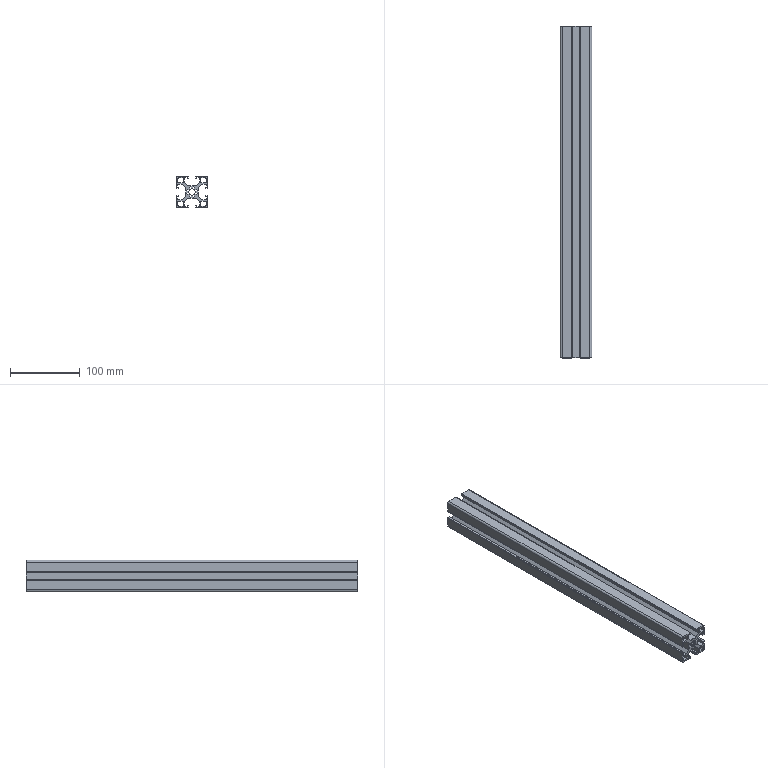Part | STEP file | 1 solid | 135 faces | box 45 x 476 x 45 mm | volume 329530 mm3 | plane 118 | cylinder 17 | commonest cylinder face diameters 10 x9 3 x4 5 x4